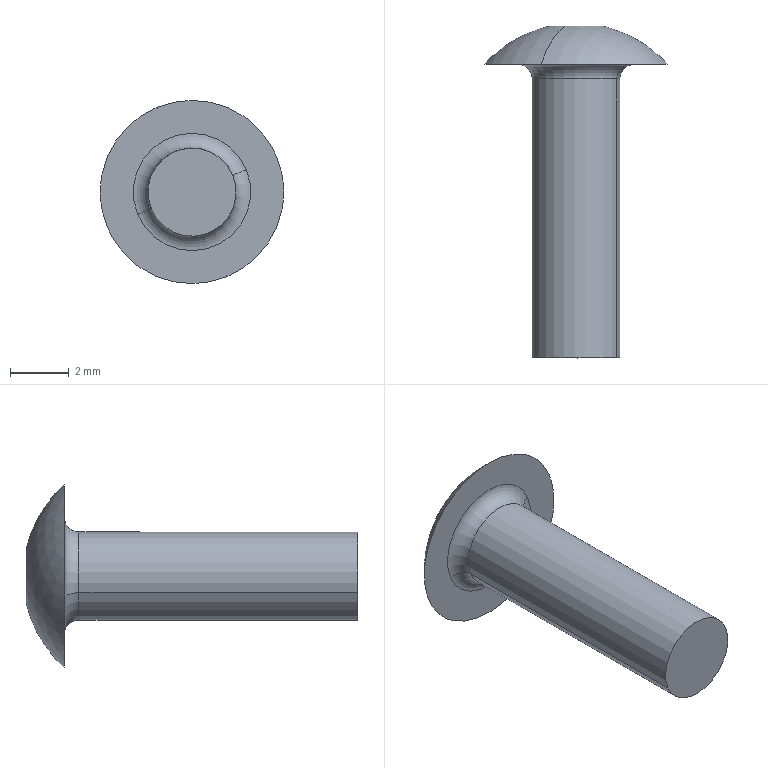Part | SolidWorks | features BaseBody 1 | 1 solid | 9 faces | box 6.24 x 11.303 x 6.24 mm | volume 93.948 mm3 | plane 3 | sphere 2 | cylinder 2 | torus 2 | commonest cylinder face diameters 3 x2
STEP:
#1=CARTESIAN_POINT('',(-251.259,16.922,-43.73));
#2=VERTEX_POINT('',#1);
#3=CARTESIAN_POINT('',(-251.958,17.843,-42.033));
#4=VERTEX_POINT('',#3);
#5=CARTESIAN_POINT('',(-252.301,13.764,-41.203));
#6=DIRECTION('',(0.9245,-0.0001344,0.3811));
#7=DIRECTION('',(0.3811,0.,-0.9245));
#8=AXIS2_PLACEMENT_3D('',#5,#6,#7);
#9=CIRCLE('',#8,4.177);
#10=EDGE_CURVE('',#2,#4,#9,.T.);
#11=ORIENTED_EDGE('',*,*,#10,.F.);
#12=CARTESIAN_POINT('',(-251.112,16.542,-44.086));
#13=VERTEX_POINT('',#12);
#14=CARTESIAN_POINT('',(-252.301,13.764,-41.203));
#15=DIRECTION('',(-0.9245,0.0001344,-0.3811));
#16=DIRECTION('',(-0.3811,0.,0.9245));
#17=AXIS2_PLACEMENT_3D('',#14,#15,#16);
#18=CIRCLE('',#17,4.177);
#19=EDGE_CURVE('',#2,#13,#18,.T.);
#20=ORIENTED_EDGE('',*,*,#19,.T.);
#21=CARTESIAN_POINT('',(-253.49,16.539,-38.317));
#22=VERTEX_POINT('',#21);
#23=CARTESIAN_POINT('',(-252.301,16.541,-41.202));
#24=DIRECTION('',(0.00003827,-1.,-0.0004455));
#25=DIRECTION('',(0.9245,-0.0001344,0.3811));
#26=AXIS2_PLACEMENT_3D('',#23,#24,#25);
#27=CIRCLE('',#26,3.12);
#28=EDGE_CURVE('',#22,#13,#27,.T.);
#29=ORIENTED_EDGE('',*,*,#28,.F.);
#30=CARTESIAN_POINT('',(-252.644,17.842,-40.369));
#31=VERTEX_POINT('',#30);
#32=CARTESIAN_POINT('',(-252.301,13.764,-41.203));
#33=DIRECTION('',(0.9245,-0.0001344,0.3811));
#34=DIRECTION('',(0.3811,0.,-0.9245));
#35=AXIS2_PLACEMENT_3D('',#32,#33,#34);
#36=CIRCLE('',#35,4.177);
#37=EDGE_CURVE('',#31,#22,#36,.T.);
#38=ORIENTED_EDGE('',*,*,#37,.F.);
#39=CARTESIAN_POINT('',(-252.301,17.842,-41.201));
#40=DIRECTION('',(-0.00003827,1.,0.0004455));
#41=DIRECTION('',(0.9245,-0.0001344,0.3811));
#42=AXIS2_PLACEMENT_3D('',#39,#40,#41);
#43=CIRCLE('',#42,0.9);
#44=EDGE_CURVE('',#4,#31,#43,.T.);
#45=ORIENTED_EDGE('',*,*,#44,.F.);
#46=EDGE_LOOP('',(#11,#20,#29,#38,#45));
#47=FACE_OUTER_BOUND('',#46,.T.);
#48=CARTESIAN_POINT('',(-252.301,13.764,-41.203));
#49=DIRECTION('',(-0.9245,0.0001344,-0.3811));
#50=DIRECTION('',(-0.288,0.6545,0.6991));
#51=AXIS2_PLACEMENT_3D('',#48,#49,#50);
#52=SPHERICAL_SURFACE('',#51,4.177);
#53=ADVANCED_FACE('',(#47),#52,.T.);
#54=CARTESIAN_POINT('',(-253.687,6.541,-41.778));
#55=VERTEX_POINT('',#54);
#56=CARTESIAN_POINT('',(-250.914,6.54,-40.635));
#57=VERTEX_POINT('',#56);
#58=CARTESIAN_POINT('',(-252.3,6.541,-41.206));
#59=DIRECTION('',(-0.00003827,1.,0.0004455));
#60=DIRECTION('',(-0.9245,0.0001344,-0.3811));
#61=AXIS2_PLACEMENT_3D('',#58,#59,#60);
#62=CIRCLE('',#61,1.5);
#63=EDGE_CURVE('',#55,#57,#62,.T.);
#64=ORIENTED_EDGE('',*,*,#63,.F.);
#65=CARTESIAN_POINT('',(-252.3,6.541,-41.206));
#66=DIRECTION('',(-0.00003827,1.,0.0004455));
#67=DIRECTION('',(0.9245,-0.0001344,0.3811));
#68=AXIS2_PLACEMENT_3D('',#65,#66,#67);
#69=CIRCLE('',#68,1.5);
#70=EDGE_CURVE('',#57,#55,#69,.T.);
#71=ORIENTED_EDGE('',*,*,#70,.F.);
#72=EDGE_LOOP('',(#64,#71));
#73=FACE_OUTER_BOUND('',#72,.T.);
#74=CARTESIAN_POINT('',(-253.132,6.541,-41.549));
#75=DIRECTION('',(-0.00003827,1.,0.0004455));
#76=DIRECTION('',(0.9963,0.,0.08559));
#77=AXIS2_PLACEMENT_3D('',#74,#75,#76);
#78=PLANE('',#77);
#79=ADVANCED_FACE('',(#73),#78,.F.);
#80=CARTESIAN_POINT('',(-253.688,16.041,-41.774));
#81=VERTEX_POINT('',#80);
#82=CARTESIAN_POINT('',(-253.688,16.041,-41.774));
#83=DIRECTION('',(0.00003827,-1.,-0.0004455));
#84=VECTOR('',#83,1000.);
#85=LINE('',#82,#84);
#86=EDGE_CURVE('',#81,#55,#85,.T.);
#87=ORIENTED_EDGE('',*,*,#86,.F.);
#88=CARTESIAN_POINT('',(-250.914,16.04,-40.63));
#89=VERTEX_POINT('',#88);
#90=CARTESIAN_POINT('',(-252.301,16.041,-41.202));
#91=DIRECTION('',(0.00003827,-1.,-0.0004455));
#92=DIRECTION('',(-0.9245,0.0001344,-0.3811));
#93=AXIS2_PLACEMENT_3D('',#90,#91,#92);
#94=CIRCLE('',#93,1.5);
#95=EDGE_CURVE('',#81,#89,#94,.T.);
#96=ORIENTED_EDGE('',*,*,#95,.T.);
#97=CARTESIAN_POINT('',(-250.914,16.04,-40.63));
#98=DIRECTION('',(0.00003827,-1.,-0.0004455));
#99=VECTOR('',#98,1000.);
#100=LINE('',#97,#99);
#101=EDGE_CURVE('',#89,#57,#100,.T.);
#102=ORIENTED_EDGE('',*,*,#101,.T.);
#103=ORIENTED_EDGE('',*,*,#70,.T.);
#104=EDGE_LOOP('',(#87,#96,#102,#103));
#105=FACE_OUTER_BOUND('',#104,.T.);
#106=CARTESIAN_POINT('',(-252.301,27.775,-41.197));
#107=DIRECTION('',(-0.00003827,1.,0.0004455));
#108=DIRECTION('',(0.9245,-0.0001344,0.3811));
#109=AXIS2_PLACEMENT_3D('',#106,#107,#108);
#110=CYLINDRICAL_SURFACE('',#109,1.5);
#111=ADVANCED_FACE('',(#105),#110,.T.);
#112=ORIENTED_EDGE('',*,*,#63,.T.);
#113=ORIENTED_EDGE('',*,*,#101,.F.);
#114=CARTESIAN_POINT('',(-252.301,16.041,-41.202));
#115=DIRECTION('',(0.00003827,-1.,-0.0004455));
#116=DIRECTION('',(0.9245,-0.0001344,0.3811));
#117=AXIS2_PLACEMENT_3D('',#114,#115,#116);
#118=CIRCLE('',#117,1.5);
#119=EDGE_CURVE('',#89,#81,#118,.T.);
#120=ORIENTED_EDGE('',*,*,#119,.T.);
#121=ORIENTED_EDGE('',*,*,#86,.T.);
#122=EDGE_LOOP('',(#112,#113,#120,#121));
#123=FACE_OUTER_BOUND('',#122,.T.);
#124=CARTESIAN_POINT('',(-252.301,27.775,-41.197));
#125=DIRECTION('',(-0.00003827,1.,0.0004455));
#126=DIRECTION('',(0.9245,-0.0001344,0.3811));
#127=AXIS2_PLACEMENT_3D('',#124,#125,#126);
#128=CYLINDRICAL_SURFACE('',#127,1.5);
#129=ADVANCED_FACE('',(#123),#128,.T.);
#130=ORIENTED_EDGE('',*,*,#119,.F.);
#131=CARTESIAN_POINT('',(-250.452,16.54,-40.44));
#132=VERTEX_POINT('',#131);
#133=CARTESIAN_POINT('',(-250.452,16.04,-40.44));
#134=DIRECTION('',(-0.3811,-0.0004264,0.9245));
#135=DIRECTION('',(-0.00003827,1.,0.0004455));
#136=AXIS2_PLACEMENT_3D('',#133,#134,#135);
#137=CIRCLE('',#136,0.5);
#138=EDGE_CURVE('',#132,#89,#137,.T.);
#139=ORIENTED_EDGE('',*,*,#138,.F.);
#140=CARTESIAN_POINT('',(-254.15,16.541,-41.964));
#141=VERTEX_POINT('',#140);
#142=CARTESIAN_POINT('',(-252.301,16.541,-41.202));
#143=DIRECTION('',(0.00003827,-1.,-0.0004455));
#144=DIRECTION('',(0.9245,-0.0001344,0.3811));
#145=AXIS2_PLACEMENT_3D('',#142,#143,#144);
#146=CIRCLE('',#145,2.);
#147=EDGE_CURVE('',#132,#141,#146,.T.);
#148=ORIENTED_EDGE('',*,*,#147,.T.);
#149=CARTESIAN_POINT('',(-254.15,16.041,-41.964));
#150=DIRECTION('',(0.3811,0.0004264,-0.9245));
#151=DIRECTION('',(-0.00003827,1.,0.0004455));
#152=AXIS2_PLACEMENT_3D('',#149,#150,#151);
#153=CIRCLE('',#152,0.5);
#154=EDGE_CURVE('',#141,#81,#153,.T.);
#155=ORIENTED_EDGE('',*,*,#154,.T.);
#156=EDGE_LOOP('',(#130,#139,#148,#155));
#157=FACE_OUTER_BOUND('',#156,.T.);
#158=CARTESIAN_POINT('',(-252.301,16.041,-41.202));
#159=DIRECTION('',(-0.00003827,1.,0.0004455));
#160=DIRECTION('',(-0.9245,0.0001344,-0.3811));
#161=AXIS2_PLACEMENT_3D('',#158,#159,#160);
#162=TOROIDAL_SURFACE('',#161,2.,0.5);
#163=ADVANCED_FACE('',(#157),#162,.F.);
#164=ORIENTED_EDGE('',*,*,#154,.F.);
#165=CARTESIAN_POINT('',(-252.301,16.541,-41.202));
#166=DIRECTION('',(0.00003827,-1.,-0.0004455));
#167=DIRECTION('',(-0.9245,0.0001344,-0.3811));
#168=AXIS2_PLACEMENT_3D('',#165,#166,#167);
#169=CIRCLE('',#168,2.);
#170=EDGE_CURVE('',#141,#132,#169,.T.);
#171=ORIENTED_EDGE('',*,*,#170,.T.);
#172=ORIENTED_EDGE('',*,*,#138,.T.);
#173=ORIENTED_EDGE('',*,*,#95,.F.);
#174=EDGE_LOOP('',(#164,#171,#172,#173));
#175=FACE_OUTER_BOUND('',#174,.T.);
#176=CARTESIAN_POINT('',(-252.301,16.041,-41.202));
#177=DIRECTION('',(-0.00003827,1.,0.0004455));
#178=DIRECTION('',(0.9245,-0.0001344,0.3811));
#179=AXIS2_PLACEMENT_3D('',#176,#177,#178);
#180=TOROIDAL_SURFACE('',#179,2.,0.5);
#181=ADVANCED_FACE('',(#175),#180,.F.);
#182=ORIENTED_EDGE('',*,*,#170,.F.);
#183=ORIENTED_EDGE('',*,*,#147,.F.);
#184=EDGE_LOOP('',(#182,#183));
#185=FACE_BOUND('',#184,.T.);
#186=ORIENTED_EDGE('',*,*,#28,.T.);
#187=CARTESIAN_POINT('',(-252.301,16.541,-41.202));
#188=DIRECTION('',(0.00003827,-1.,-0.0004455));
#189=DIRECTION('',(0.9245,-0.0001344,0.3811));
#190=AXIS2_PLACEMENT_3D('',#187,#188,#189);
#191=CIRCLE('',#190,3.12);
#192=EDGE_CURVE('',#13,#22,#191,.T.);
#193=ORIENTED_EDGE('',*,*,#192,.T.);
#194=EDGE_LOOP('',(#186,#193));
#195=FACE_OUTER_BOUND('',#194,.T.);
#196=CARTESIAN_POINT('',(-253.688,16.541,-41.773));
#197=DIRECTION('',(-0.00003827,1.,0.0004455));
#198=DIRECTION('',(0.9963,0.,0.08559));
#199=AXIS2_PLACEMENT_3D('',#196,#197,#198);
#200=PLANE('',#199);
#201=ADVANCED_FACE('',(#185,#195),#200,.F.);
#202=ORIENTED_EDGE('',*,*,#19,.F.);
#203=ORIENTED_EDGE('',*,*,#10,.T.);
#204=CARTESIAN_POINT('',(-252.301,17.842,-41.201));
#205=DIRECTION('',(-0.00003827,1.,0.0004455));
#206=DIRECTION('',(0.9245,-0.0001344,0.3811));
#207=AXIS2_PLACEMENT_3D('',#204,#205,#206);
#208=CIRCLE('',#207,0.9);
#209=EDGE_CURVE('',#31,#4,#208,.T.);
#210=ORIENTED_EDGE('',*,*,#209,.F.);
#211=ORIENTED_EDGE('',*,*,#37,.T.);
#212=ORIENTED_EDGE('',*,*,#192,.F.);
#213=EDGE_LOOP('',(#202,#203,#210,#211,#212));
#214=FACE_OUTER_BOUND('',#213,.T.);
#215=CARTESIAN_POINT('',(-252.301,13.764,-41.203));
#216=DIRECTION('',(-0.9245,0.0001344,-0.3811));
#217=DIRECTION('',(-0.288,0.6545,0.6991));
#218=AXIS2_PLACEMENT_3D('',#215,#216,#217);
#219=SPHERICAL_SURFACE('',#218,4.177);
#220=ADVANCED_FACE('',(#214),#219,.T.);
#221=ORIENTED_EDGE('',*,*,#44,.T.);
#222=ORIENTED_EDGE('',*,*,#209,.T.);
#223=EDGE_LOOP('',(#221,#222));
#224=FACE_OUTER_BOUND('',#223,.T.);
#225=CARTESIAN_POINT('',(-252.301,17.842,-41.201));
#226=DIRECTION('',(-0.00003827,1.,0.0004455));
#227=DIRECTION('',(0.9963,0.,0.08559));
#228=AXIS2_PLACEMENT_3D('',#225,#226,#227);
#229=PLANE('',#228);
#230=ADVANCED_FACE('',(#224),#229,.T.);
#231=CLOSED_SHELL('',(#53,#79,#111,#129,#163,#181,#201,#220,#230));
#232=MANIFOLD_SOLID_BREP('',#231);
#233=CARTESIAN_POINT('',(0.,0.,0.));
#234=DIRECTION('',(0.,0.,1.));
#235=DIRECTION('',(1.,0.,0.));
#236=AXIS2_PLACEMENT_3D('',#233,#234,#235);
#237=(LENGTH_UNIT()NAMED_UNIT(*)SI_UNIT(.MILLI.,.METRE.));
#238=UNCERTAINTY_MEASURE_WITH_UNIT(LENGTH_MEASURE(0.00001),#237,'','');
#239=(NAMED_UNIT(*)PLANE_ANGLE_UNIT()SI_UNIT($,.RADIAN.));
#240=(NAMED_UNIT(*)SI_UNIT($,.STERADIAN.)SOLID_ANGLE_UNIT());
#241=(GEOMETRIC_REPRESENTATION_CONTEXT(3)GLOBAL_UNCERTAINTY_ASSIGNED_CONTEXT((#238))GLOBAL_UNIT_ASSIGNED_CONTEXT((#237,#239,#240))REPRESENTATION_CONTEXT('',''));
#242=ADVANCED_BREP_SHAPE_REPRESENTATION('',(#232,#236),#241);